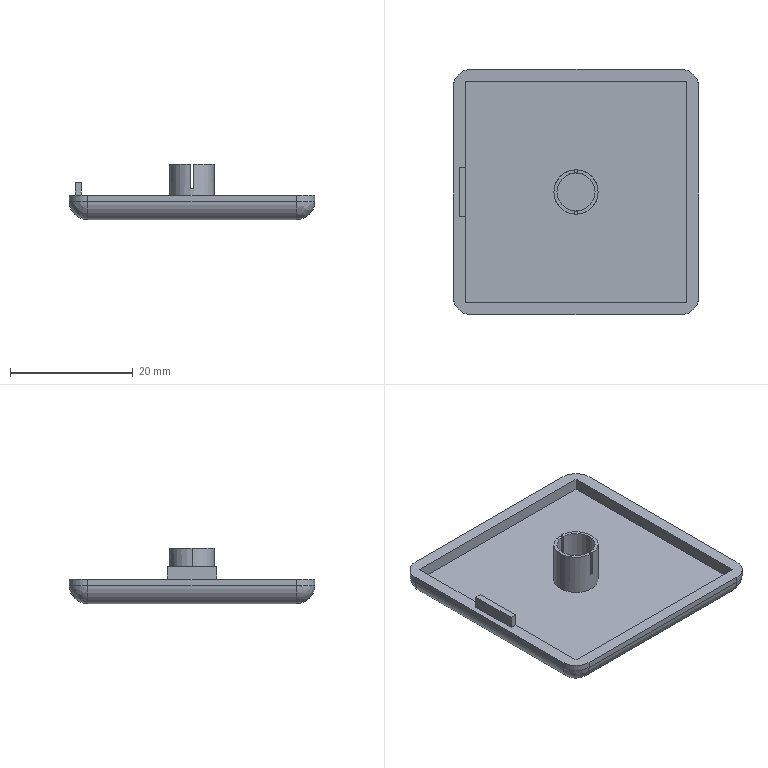Part | SolidWorks | features BaseBody 1 | 1 solid | 40 faces | box 40 x 40 x 9 mm | volume 3574 mm3 | plane 24 | cylinder 12 | spline 4 | commonest cylinder face diameters 6 x8 6.2 x2 7.2 x2
STEP:
#1=CARTESIAN_POINT('',(3.6,0.,-2.));
#2=VERTEX_POINT('',#1);
#3=CARTESIAN_POINT('',(-3.6,0.,-2.));
#4=VERTEX_POINT('',#3);
#5=CARTESIAN_POINT('',(0.,0.,-2.));
#6=DIRECTION('',(0.,0.,-1.));
#7=DIRECTION('',(-1.,0.,0.));
#8=AXIS2_PLACEMENT_3D('',#5,#6,#7);
#9=CIRCLE('',#8,3.6);
#10=EDGE_CURVE('',#2,#4,#9,.T.);
#11=ORIENTED_EDGE('',*,*,#10,.F.);
#12=CARTESIAN_POINT('',(3.6,0.,5.));
#13=VERTEX_POINT('',#12);
#14=CARTESIAN_POINT('',(3.6,0.,5.));
#15=DIRECTION('',(0.,0.,1.));
#16=VECTOR('',#15,1000.);
#17=LINE('',#14,#16);
#18=EDGE_CURVE('',#2,#13,#17,.T.);
#19=ORIENTED_EDGE('',*,*,#18,.T.);
#20=CARTESIAN_POINT('',(0.288,-3.588,5.));
#21=VERTEX_POINT('',#20);
#22=CARTESIAN_POINT('',(0.,0.,5.));
#23=DIRECTION('',(0.,0.,-1.));
#24=DIRECTION('',(-1.,0.,0.));
#25=AXIS2_PLACEMENT_3D('',#22,#23,#24);
#26=CIRCLE('',#25,3.6);
#27=EDGE_CURVE('',#13,#21,#26,.T.);
#28=ORIENTED_EDGE('',*,*,#27,.T.);
#29=CARTESIAN_POINT('',(0.288,-3.588,1.));
#30=VERTEX_POINT('',#29);
#31=CARTESIAN_POINT('',(0.288,-3.588,5.));
#32=DIRECTION('',(0.,0.,-1.));
#33=VECTOR('',#32,1000.);
#34=LINE('',#31,#33);
#35=EDGE_CURVE('',#21,#30,#34,.T.);
#36=ORIENTED_EDGE('',*,*,#35,.T.);
#37=CARTESIAN_POINT('',(-0.288,-3.588,1.));
#38=VERTEX_POINT('',#37);
#39=CARTESIAN_POINT('',(0.,0.,1.));
#40=DIRECTION('',(0.,0.,-1.));
#41=DIRECTION('',(-1.,0.,0.));
#42=AXIS2_PLACEMENT_3D('',#39,#40,#41);
#43=CIRCLE('',#42,3.6);
#44=EDGE_CURVE('',#30,#38,#43,.T.);
#45=ORIENTED_EDGE('',*,*,#44,.T.);
#46=CARTESIAN_POINT('',(-0.288,-3.588,5.));
#47=VERTEX_POINT('',#46);
#48=CARTESIAN_POINT('',(-0.288,-3.588,5.));
#49=DIRECTION('',(0.,0.,1.));
#50=VECTOR('',#49,1000.);
#51=LINE('',#48,#50);
#52=EDGE_CURVE('',#38,#47,#51,.T.);
#53=ORIENTED_EDGE('',*,*,#52,.T.);
#54=CARTESIAN_POINT('',(-3.6,0.,5.));
#55=VERTEX_POINT('',#54);
#56=CARTESIAN_POINT('',(0.,0.,5.));
#57=DIRECTION('',(0.,0.,-1.));
#58=DIRECTION('',(-1.,0.,0.));
#59=AXIS2_PLACEMENT_3D('',#56,#57,#58);
#60=CIRCLE('',#59,3.6);
#61=EDGE_CURVE('',#47,#55,#60,.T.);
#62=ORIENTED_EDGE('',*,*,#61,.T.);
#63=CARTESIAN_POINT('',(-3.6,0.,5.));
#64=DIRECTION('',(0.,0.,1.));
#65=VECTOR('',#64,1000.);
#66=LINE('',#63,#65);
#67=EDGE_CURVE('',#4,#55,#66,.T.);
#68=ORIENTED_EDGE('',*,*,#67,.F.);
#69=EDGE_LOOP('',(#11,#19,#28,#36,#45,#53,#62,#68));
#70=FACE_OUTER_BOUND('',#69,.T.);
#71=CARTESIAN_POINT('',(0.,0.,5.));
#72=DIRECTION('',(0.,0.,1.));
#73=DIRECTION('',(-1.,0.,0.));
#74=AXIS2_PLACEMENT_3D('',#71,#72,#73);
#75=CYLINDRICAL_SURFACE('',#74,3.6);
#76=ADVANCED_FACE('',(#70),#75,.T.);
#77=CARTESIAN_POINT('',(3.1,0.,-2.));
#78=VERTEX_POINT('',#77);
#79=CARTESIAN_POINT('',(-3.1,0.,-2.));
#80=VERTEX_POINT('',#79);
#81=CARTESIAN_POINT('',(0.,0.,-2.));
#82=DIRECTION('',(0.,0.,1.));
#83=DIRECTION('',(-1.,0.,0.));
#84=AXIS2_PLACEMENT_3D('',#81,#82,#83);
#85=CIRCLE('',#84,3.1);
#86=EDGE_CURVE('',#78,#80,#85,.T.);
#87=ORIENTED_EDGE('',*,*,#86,.F.);
#88=CARTESIAN_POINT('',(3.1,0.,5.));
#89=VERTEX_POINT('',#88);
#90=CARTESIAN_POINT('',(3.1,0.,5.));
#91=DIRECTION('',(0.,0.,1.));
#92=VECTOR('',#91,1000.);
#93=LINE('',#90,#92);
#94=EDGE_CURVE('',#78,#89,#93,.T.);
#95=ORIENTED_EDGE('',*,*,#94,.T.);
#96=CARTESIAN_POINT('',(0.288,3.087,5.));
#97=VERTEX_POINT('',#96);
#98=CARTESIAN_POINT('',(0.,0.,5.));
#99=DIRECTION('',(0.,0.,-1.));
#100=DIRECTION('',(-1.,0.,0.));
#101=AXIS2_PLACEMENT_3D('',#98,#99,#100);
#102=CIRCLE('',#101,3.1);
#103=EDGE_CURVE('',#97,#89,#102,.T.);
#104=ORIENTED_EDGE('',*,*,#103,.F.);
#105=CARTESIAN_POINT('',(0.288,3.087,1.));
#106=VERTEX_POINT('',#105);
#107=CARTESIAN_POINT('',(0.288,3.087,1.));
#108=DIRECTION('',(0.,0.,-1.));
#109=VECTOR('',#108,1000.);
#110=LINE('',#107,#109);
#111=EDGE_CURVE('',#97,#106,#110,.T.);
#112=ORIENTED_EDGE('',*,*,#111,.T.);
#113=CARTESIAN_POINT('',(-0.288,3.087,1.));
#114=VERTEX_POINT('',#113);
#115=CARTESIAN_POINT('',(0.,0.,1.));
#116=DIRECTION('',(0.,0.,-1.));
#117=DIRECTION('',(-1.,0.,0.));
#118=AXIS2_PLACEMENT_3D('',#115,#116,#117);
#119=CIRCLE('',#118,3.1);
#120=EDGE_CURVE('',#114,#106,#119,.T.);
#121=ORIENTED_EDGE('',*,*,#120,.F.);
#122=CARTESIAN_POINT('',(-0.288,3.087,5.));
#123=VERTEX_POINT('',#122);
#124=CARTESIAN_POINT('',(-0.288,3.087,1.));
#125=DIRECTION('',(0.,0.,1.));
#126=VECTOR('',#125,1000.);
#127=LINE('',#124,#126);
#128=EDGE_CURVE('',#114,#123,#127,.T.);
#129=ORIENTED_EDGE('',*,*,#128,.T.);
#130=CARTESIAN_POINT('',(-3.1,0.,5.));
#131=VERTEX_POINT('',#130);
#132=CARTESIAN_POINT('',(0.,0.,5.));
#133=DIRECTION('',(0.,0.,-1.));
#134=DIRECTION('',(-1.,0.,0.));
#135=AXIS2_PLACEMENT_3D('',#132,#133,#134);
#136=CIRCLE('',#135,3.1);
#137=EDGE_CURVE('',#131,#123,#136,.T.);
#138=ORIENTED_EDGE('',*,*,#137,.F.);
#139=CARTESIAN_POINT('',(-3.1,0.,5.));
#140=DIRECTION('',(0.,0.,1.));
#141=VECTOR('',#140,1000.);
#142=LINE('',#139,#141);
#143=EDGE_CURVE('',#80,#131,#142,.T.);
#144=ORIENTED_EDGE('',*,*,#143,.F.);
#145=EDGE_LOOP('',(#87,#95,#104,#112,#121,#129,#138,#144));
#146=FACE_OUTER_BOUND('',#145,.T.);
#147=CARTESIAN_POINT('',(0.,0.,5.));
#148=DIRECTION('',(0.,0.,1.));
#149=DIRECTION('',(-1.,0.,0.));
#150=AXIS2_PLACEMENT_3D('',#147,#148,#149);
#151=CYLINDRICAL_SURFACE('',#150,3.1);
#152=ADVANCED_FACE('',(#146),#151,.F.);
#153=CARTESIAN_POINT('',(-18.,-18.,-2.));
#154=VERTEX_POINT('',#153);
#155=CARTESIAN_POINT('',(18.,-18.,-2.));
#156=VERTEX_POINT('',#155);
#157=CARTESIAN_POINT('',(-20.,-18.,-2.));
#158=DIRECTION('',(1.,0.,0.));
#159=VECTOR('',#158,1000.);
#160=LINE('',#157,#159);
#161=EDGE_CURVE('',#154,#156,#160,.T.);
#162=ORIENTED_EDGE('',*,*,#161,.T.);
#163=CARTESIAN_POINT('',(18.,18.,-2.));
#164=VERTEX_POINT('',#163);
#165=CARTESIAN_POINT('',(18.,20.,-2.));
#166=DIRECTION('',(0.,1.,0.));
#167=VECTOR('',#166,1000.);
#168=LINE('',#165,#167);
#169=EDGE_CURVE('',#156,#164,#168,.T.);
#170=ORIENTED_EDGE('',*,*,#169,.T.);
#171=CARTESIAN_POINT('',(-18.,18.,-2.));
#172=VERTEX_POINT('',#171);
#173=CARTESIAN_POINT('',(-20.,18.,-2.));
#174=DIRECTION('',(-1.,0.,0.));
#175=VECTOR('',#174,1000.);
#176=LINE('',#173,#175);
#177=EDGE_CURVE('',#164,#172,#176,.T.);
#178=ORIENTED_EDGE('',*,*,#177,.T.);
#179=CARTESIAN_POINT('',(-18.,20.,-2.));
#180=DIRECTION('',(0.,-1.,0.));
#181=VECTOR('',#180,1000.);
#182=LINE('',#179,#181);
#183=EDGE_CURVE('',#172,#154,#182,.T.);
#184=ORIENTED_EDGE('',*,*,#183,.T.);
#185=EDGE_LOOP('',(#162,#170,#178,#184));
#186=FACE_OUTER_BOUND('',#185,.T.);
#187=CARTESIAN_POINT('',(0.,0.,-2.));
#188=DIRECTION('',(0.,0.,-1.));
#189=DIRECTION('',(-1.,0.,0.));
#190=AXIS2_PLACEMENT_3D('',#187,#188,#189);
#191=CIRCLE('',#190,3.6);
#192=EDGE_CURVE('',#4,#2,#191,.T.);
#193=ORIENTED_EDGE('',*,*,#192,.T.);
#194=ORIENTED_EDGE('',*,*,#10,.T.);
#195=EDGE_LOOP('',(#193,#194));
#196=FACE_BOUND('',#195,.T.);
#197=CARTESIAN_POINT('',(-20.,20.,-2.));
#198=DIRECTION('',(0.,0.,1.));
#199=DIRECTION('',(-1.,0.,0.));
#200=AXIS2_PLACEMENT_3D('',#197,#198,#199);
#201=PLANE('',#200);
#202=ADVANCED_FACE('',(#186,#196),#201,.T.);
#203=CARTESIAN_POINT('',(18.,18.,0.));
#204=VERTEX_POINT('',#203);
#205=CARTESIAN_POINT('',(18.,18.,-2.));
#206=DIRECTION('',(0.,0.,1.));
#207=VECTOR('',#206,1000.);
#208=LINE('',#205,#207);
#209=EDGE_CURVE('',#164,#204,#208,.T.);
#210=ORIENTED_EDGE('',*,*,#209,.F.);
#211=ORIENTED_EDGE('',*,*,#169,.F.);
#212=CARTESIAN_POINT('',(18.,-18.,0.));
#213=VERTEX_POINT('',#212);
#214=CARTESIAN_POINT('',(18.,-18.,-2.));
#215=DIRECTION('',(0.,0.,-1.));
#216=VECTOR('',#215,1000.);
#217=LINE('',#214,#216);
#218=EDGE_CURVE('',#213,#156,#217,.T.);
#219=ORIENTED_EDGE('',*,*,#218,.F.);
#220=CARTESIAN_POINT('',(18.,-18.,0.));
#221=DIRECTION('',(0.,-1.,0.));
#222=VECTOR('',#221,1000.);
#223=LINE('',#220,#222);
#224=EDGE_CURVE('',#204,#213,#223,.T.);
#225=ORIENTED_EDGE('',*,*,#224,.F.);
#226=EDGE_LOOP('',(#210,#211,#219,#225));
#227=FACE_OUTER_BOUND('',#226,.T.);
#228=CARTESIAN_POINT('',(18.,-18.,-2.));
#229=DIRECTION('',(1.,0.,0.));
#230=DIRECTION('',(0.,1.,0.));
#231=AXIS2_PLACEMENT_3D('',#228,#229,#230);
#232=PLANE('',#231);
#233=ADVANCED_FACE('',(#227),#232,.F.);
#234=ORIENTED_EDGE('',*,*,#218,.T.);
#235=ORIENTED_EDGE('',*,*,#161,.F.);
#236=CARTESIAN_POINT('',(-18.,-18.,0.));
#237=VERTEX_POINT('',#236);
#238=CARTESIAN_POINT('',(-18.,-18.,-2.));
#239=DIRECTION('',(0.,0.,-1.));
#240=VECTOR('',#239,1000.);
#241=LINE('',#238,#240);
#242=EDGE_CURVE('',#237,#154,#241,.T.);
#243=ORIENTED_EDGE('',*,*,#242,.F.);
#244=CARTESIAN_POINT('',(-18.,-18.,0.));
#245=DIRECTION('',(-1.,0.,0.));
#246=VECTOR('',#245,1000.);
#247=LINE('',#244,#246);
#248=EDGE_CURVE('',#213,#237,#247,.T.);
#249=ORIENTED_EDGE('',*,*,#248,.F.);
#250=EDGE_LOOP('',(#234,#235,#243,#249));
#251=FACE_OUTER_BOUND('',#250,.T.);
#252=CARTESIAN_POINT('',(-18.,-18.,-2.));
#253=DIRECTION('',(0.,-1.,0.));
#254=DIRECTION('',(1.,0.,0.));
#255=AXIS2_PLACEMENT_3D('',#252,#253,#254);
#256=PLANE('',#255);
#257=ADVANCED_FACE('',(#251),#256,.F.);
#258=CARTESIAN_POINT('',(-18.,4.05,2.));
#259=VERTEX_POINT('',#258);
#260=CARTESIAN_POINT('',(-18.,4.05,0.));
#261=VERTEX_POINT('',#260);
#262=CARTESIAN_POINT('',(-18.,4.05,-2.));
#263=DIRECTION('',(0.,0.,-1.));
#264=VECTOR('',#263,1000.);
#265=LINE('',#262,#264);
#266=EDGE_CURVE('',#259,#261,#265,.T.);
#267=ORIENTED_EDGE('',*,*,#266,.F.);
#268=CARTESIAN_POINT('',(-18.,-4.05,2.));
#269=VERTEX_POINT('',#268);
#270=CARTESIAN_POINT('',(-18.,18.,2.));
#271=DIRECTION('',(0.,1.,0.));
#272=VECTOR('',#271,1000.);
#273=LINE('',#270,#272);
#274=EDGE_CURVE('',#269,#259,#273,.T.);
#275=ORIENTED_EDGE('',*,*,#274,.F.);
#276=CARTESIAN_POINT('',(-18.,-4.05,0.));
#277=VERTEX_POINT('',#276);
#278=CARTESIAN_POINT('',(-18.,-4.05,-2.));
#279=DIRECTION('',(0.,0.,1.));
#280=VECTOR('',#279,1000.);
#281=LINE('',#278,#280);
#282=EDGE_CURVE('',#277,#269,#281,.T.);
#283=ORIENTED_EDGE('',*,*,#282,.F.);
#284=CARTESIAN_POINT('',(-18.,18.,0.));
#285=DIRECTION('',(0.,1.,0.));
#286=VECTOR('',#285,1000.);
#287=LINE('',#284,#286);
#288=EDGE_CURVE('',#237,#277,#287,.T.);
#289=ORIENTED_EDGE('',*,*,#288,.F.);
#290=ORIENTED_EDGE('',*,*,#242,.T.);
#291=ORIENTED_EDGE('',*,*,#183,.F.);
#292=CARTESIAN_POINT('',(-18.,18.,0.));
#293=VERTEX_POINT('',#292);
#294=CARTESIAN_POINT('',(-18.,18.,-2.));
#295=DIRECTION('',(0.,0.,-1.));
#296=VECTOR('',#295,1000.);
#297=LINE('',#294,#296);
#298=EDGE_CURVE('',#293,#172,#297,.T.);
#299=ORIENTED_EDGE('',*,*,#298,.F.);
#300=CARTESIAN_POINT('',(-18.,18.,0.));
#301=DIRECTION('',(0.,1.,0.));
#302=VECTOR('',#301,1000.);
#303=LINE('',#300,#302);
#304=EDGE_CURVE('',#261,#293,#303,.T.);
#305=ORIENTED_EDGE('',*,*,#304,.F.);
#306=EDGE_LOOP('',(#267,#275,#283,#289,#290,#291,#299,#305));
#307=FACE_OUTER_BOUND('',#306,.T.);
#308=CARTESIAN_POINT('',(-18.,18.,-2.));
#309=DIRECTION('',(-1.,0.,0.));
#310=DIRECTION('',(0.,-1.,0.));
#311=AXIS2_PLACEMENT_3D('',#308,#309,#310);
#312=PLANE('',#311);
#313=ADVANCED_FACE('',(#307),#312,.F.);
#314=ORIENTED_EDGE('',*,*,#298,.T.);
#315=ORIENTED_EDGE('',*,*,#177,.F.);
#316=ORIENTED_EDGE('',*,*,#209,.T.);
#317=CARTESIAN_POINT('',(18.,18.,0.));
#318=DIRECTION('',(1.,0.,0.));
#319=VECTOR('',#318,1000.);
#320=LINE('',#317,#319);
#321=EDGE_CURVE('',#293,#204,#320,.T.);
#322=ORIENTED_EDGE('',*,*,#321,.F.);
#323=EDGE_LOOP('',(#314,#315,#316,#322));
#324=FACE_OUTER_BOUND('',#323,.T.);
#325=CARTESIAN_POINT('',(18.,18.,-2.));
#326=DIRECTION('',(0.,1.,0.));
#327=DIRECTION('',(-1.,0.,0.));
#328=AXIS2_PLACEMENT_3D('',#325,#326,#327);
#329=PLANE('',#328);
#330=ADVANCED_FACE('',(#324),#329,.F.);
#331=ORIENTED_EDGE('',*,*,#18,.F.);
#332=ORIENTED_EDGE('',*,*,#192,.F.);
#333=ORIENTED_EDGE('',*,*,#67,.T.);
#334=CARTESIAN_POINT('',(-0.288,3.588,5.));
#335=VERTEX_POINT('',#334);
#336=CARTESIAN_POINT('',(0.,0.,5.));
#337=DIRECTION('',(0.,0.,-1.));
#338=DIRECTION('',(-1.,0.,0.));
#339=AXIS2_PLACEMENT_3D('',#336,#337,#338);
#340=CIRCLE('',#339,3.6);
#341=EDGE_CURVE('',#55,#335,#340,.T.);
#342=ORIENTED_EDGE('',*,*,#341,.T.);
#343=CARTESIAN_POINT('',(-0.288,3.588,1.));
#344=VERTEX_POINT('',#343);
#345=CARTESIAN_POINT('',(-0.288,3.588,5.));
#346=DIRECTION('',(0.,0.,-1.));
#347=VECTOR('',#346,1000.);
#348=LINE('',#345,#347);
#349=EDGE_CURVE('',#335,#344,#348,.T.);
#350=ORIENTED_EDGE('',*,*,#349,.T.);
#351=CARTESIAN_POINT('',(0.288,3.588,1.));
#352=VERTEX_POINT('',#351);
#353=CARTESIAN_POINT('',(0.,0.,1.));
#354=DIRECTION('',(0.,0.,-1.));
#355=DIRECTION('',(-1.,0.,0.));
#356=AXIS2_PLACEMENT_3D('',#353,#354,#355);
#357=CIRCLE('',#356,3.6);
#358=EDGE_CURVE('',#344,#352,#357,.T.);
#359=ORIENTED_EDGE('',*,*,#358,.T.);
#360=CARTESIAN_POINT('',(0.288,3.588,5.));
#361=VERTEX_POINT('',#360);
#362=CARTESIAN_POINT('',(0.288,3.588,5.));
#363=DIRECTION('',(0.,0.,1.));
#364=VECTOR('',#363,1000.);
#365=LINE('',#362,#364);
#366=EDGE_CURVE('',#352,#361,#365,.T.);
#367=ORIENTED_EDGE('',*,*,#366,.T.);
#368=CARTESIAN_POINT('',(0.,0.,5.));
#369=DIRECTION('',(0.,0.,-1.));
#370=DIRECTION('',(-1.,0.,0.));
#371=AXIS2_PLACEMENT_3D('',#368,#369,#370);
#372=CIRCLE('',#371,3.6);
#373=EDGE_CURVE('',#361,#13,#372,.T.);
#374=ORIENTED_EDGE('',*,*,#373,.T.);
#375=EDGE_LOOP('',(#331,#332,#333,#342,#350,#359,#367,#374));
#376=FACE_OUTER_BOUND('',#375,.T.);
#377=CARTESIAN_POINT('',(0.,0.,5.));
#378=DIRECTION('',(0.,0.,1.));
#379=DIRECTION('',(-1.,0.,0.));
#380=AXIS2_PLACEMENT_3D('',#377,#378,#379);
#381=CYLINDRICAL_SURFACE('',#380,3.6);
#382=ADVANCED_FACE('',(#376),#381,.T.);
#383=CARTESIAN_POINT('',(20.,-17.,0.));
#384=VERTEX_POINT('',#383);
#385=CARTESIAN_POINT('',(20.,17.,0.));
#386=VERTEX_POINT('',#385);
#387=CARTESIAN_POINT('',(20.,17.,0.));
#388=DIRECTION('',(0.,1.,0.));
#389=VECTOR('',#388,1000.);
#390=LINE('',#387,#389);
#391=EDGE_CURVE('',#384,#386,#390,.T.);
#392=ORIENTED_EDGE('',*,*,#391,.T.);
#393=CARTESIAN_POINT('',(17.,20.,0.));
#394=VERTEX_POINT('',#393);
#395=CARTESIAN_POINT('',(17.,17.,0.));
#396=DIRECTION('',(0.,0.,1.));
#397=DIRECTION('',(1.,0.,0.));
#398=AXIS2_PLACEMENT_3D('',#395,#396,#397);
#399=CIRCLE('',#398,3.);
#400=EDGE_CURVE('',#386,#394,#399,.T.);
#401=ORIENTED_EDGE('',*,*,#400,.T.);
#402=CARTESIAN_POINT('',(-17.,20.,0.));
#403=VERTEX_POINT('',#402);
#404=CARTESIAN_POINT('',(-17.,20.,0.));
#405=DIRECTION('',(-1.,0.,0.));
#406=VECTOR('',#405,1000.);
#407=LINE('',#404,#406);
#408=EDGE_CURVE('',#394,#403,#407,.T.);
#409=ORIENTED_EDGE('',*,*,#408,.T.);
#410=CARTESIAN_POINT('',(-20.,17.,0.));
#411=VERTEX_POINT('',#410);
#412=CARTESIAN_POINT('',(-17.,17.,0.));
#413=DIRECTION('',(0.,0.,1.));
#414=DIRECTION('',(1.,0.,0.));
#415=AXIS2_PLACEMENT_3D('',#412,#413,#414);
#416=CIRCLE('',#415,3.);
#417=EDGE_CURVE('',#403,#411,#416,.T.);
#418=ORIENTED_EDGE('',*,*,#417,.T.);
#419=CARTESIAN_POINT('',(-20.,-17.,0.));
#420=VERTEX_POINT('',#419);
#421=CARTESIAN_POINT('',(-20.,17.,0.));
#422=DIRECTION('',(0.,-1.,0.));
#423=VECTOR('',#422,1000.);
#424=LINE('',#421,#423);
#425=EDGE_CURVE('',#411,#420,#424,.T.);
#426=ORIENTED_EDGE('',*,*,#425,.T.);
#427=CARTESIAN_POINT('',(-17.,-20.,0.));
#428=VERTEX_POINT('',#427);
#429=CARTESIAN_POINT('',(-17.,-17.,0.));
#430=DIRECTION('',(0.,0.,1.));
#431=DIRECTION('',(1.,0.,0.));
#432=AXIS2_PLACEMENT_3D('',#429,#430,#431);
#433=CIRCLE('',#432,3.);
#434=EDGE_CURVE('',#420,#428,#433,.T.);
#435=ORIENTED_EDGE('',*,*,#434,.T.);
#436=CARTESIAN_POINT('',(17.,-20.,0.));
#437=VERTEX_POINT('',#436);
#438=CARTESIAN_POINT('',(-17.,-20.,0.));
#439=DIRECTION('',(1.,0.,0.));
#440=VECTOR('',#439,1000.);
#441=LINE('',#438,#440);
#442=EDGE_CURVE('',#428,#437,#441,.T.);
#443=ORIENTED_EDGE('',*,*,#442,.T.);
#444=CARTESIAN_POINT('',(17.,-17.,0.));
#445=DIRECTION('',(0.,0.,1.));
#446=DIRECTION('',(1.,0.,0.));
#447=AXIS2_PLACEMENT_3D('',#444,#445,#446);
#448=CIRCLE('',#447,3.);
#449=EDGE_CURVE('',#437,#384,#448,.T.);
#450=ORIENTED_EDGE('',*,*,#449,.T.);
#451=EDGE_LOOP('',(#392,#401,#409,#418,#426,#435,#443,#450));
#452=FACE_OUTER_BOUND('',#451,.T.);
#453=CARTESIAN_POINT('',(-19.,-4.05,0.));
#454=VERTEX_POINT('',#453);
#455=CARTESIAN_POINT('',(-17.,-4.05,0.));
#456=DIRECTION('',(-1.,0.,0.));
#457=VECTOR('',#456,1000.);
#458=LINE('',#455,#457);
#459=EDGE_CURVE('',#277,#454,#458,.T.);
#460=ORIENTED_EDGE('',*,*,#459,.T.);
#461=CARTESIAN_POINT('',(-19.,4.05,0.));
#462=VERTEX_POINT('',#461);
#463=CARTESIAN_POINT('',(-19.,17.,0.));
#464=DIRECTION('',(0.,1.,0.));
#465=VECTOR('',#464,1000.);
#466=LINE('',#463,#465);
#467=EDGE_CURVE('',#454,#462,#466,.T.);
#468=ORIENTED_EDGE('',*,*,#467,.T.);
#469=CARTESIAN_POINT('',(-17.,4.05,0.));
#470=DIRECTION('',(1.,0.,0.));
#471=VECTOR('',#470,1000.);
#472=LINE('',#469,#471);
#473=EDGE_CURVE('',#462,#261,#472,.T.);
#474=ORIENTED_EDGE('',*,*,#473,.T.);
#475=ORIENTED_EDGE('',*,*,#304,.T.);
#476=ORIENTED_EDGE('',*,*,#321,.T.);
#477=ORIENTED_EDGE('',*,*,#224,.T.);
#478=ORIENTED_EDGE('',*,*,#248,.T.);
#479=ORIENTED_EDGE('',*,*,#288,.T.);
#480=EDGE_LOOP('',(#460,#468,#474,#475,#476,#477,#478,#479));
#481=FACE_BOUND('',#480,.T.);
#482=CARTESIAN_POINT('',(-17.,17.,0.));
#483=DIRECTION('',(0.,0.,1.));
#484=DIRECTION('',(-1.,0.,0.));
#485=AXIS2_PLACEMENT_3D('',#482,#483,#484);
#486=PLANE('',#485);
#487=ADVANCED_FACE('',(#452,#481),#486,.T.);
#488=CARTESIAN_POINT('',(-19.,4.05,2.));
#489=VERTEX_POINT('',#488);
#490=CARTESIAN_POINT('',(-19.,4.05,2.));
#491=DIRECTION('',(0.,0.,-1.));
#492=VECTOR('',#491,1000.);
#493=LINE('',#490,#492);
#494=EDGE_CURVE('',#489,#462,#493,.T.);
#495=ORIENTED_EDGE('',*,*,#494,.F.);
#496=CARTESIAN_POINT('',(-18.,4.05,2.));
#497=DIRECTION('',(-1.,0.,0.));
#498=VECTOR('',#497,1000.);
#499=LINE('',#496,#498);
#500=EDGE_CURVE('',#259,#489,#499,.T.);
#501=ORIENTED_EDGE('',*,*,#500,.F.);
#502=ORIENTED_EDGE('',*,*,#266,.T.);
#503=ORIENTED_EDGE('',*,*,#473,.F.);
#504=EDGE_LOOP('',(#495,#501,#502,#503));
#505=FACE_OUTER_BOUND('',#504,.T.);
#506=CARTESIAN_POINT('',(-18.,4.05,2.));
#507=DIRECTION('',(0.,-1.,0.));
#508=DIRECTION('',(1.,0.,0.));
#509=AXIS2_PLACEMENT_3D('',#506,#507,#508);
#510=PLANE('',#509);
#511=ADVANCED_FACE('',(#505),#510,.F.);
#512=CARTESIAN_POINT('',(-19.,-4.05,2.));
#513=VERTEX_POINT('',#512);
#514=CARTESIAN_POINT('',(-20.,-4.05,2.));
#515=DIRECTION('',(1.,0.,0.));
#516=VECTOR('',#515,1000.);
#517=LINE('',#514,#516);
#518=EDGE_CURVE('',#513,#269,#517,.T.);
#519=ORIENTED_EDGE('',*,*,#518,.T.);
#520=ORIENTED_EDGE('',*,*,#274,.T.);
#521=ORIENTED_EDGE('',*,*,#500,.T.);
#522=CARTESIAN_POINT('',(-19.,20.,2.));
#523=DIRECTION('',(0.,-1.,0.));
#524=VECTOR('',#523,1000.);
#525=LINE('',#522,#524);
#526=EDGE_CURVE('',#489,#513,#525,.T.);
#527=ORIENTED_EDGE('',*,*,#526,.T.);
#528=EDGE_LOOP('',(#519,#520,#521,#527));
#529=FACE_OUTER_BOUND('',#528,.T.);
#530=CARTESIAN_POINT('',(-20.,20.,2.));
#531=DIRECTION('',(0.,0.,1.));
#532=DIRECTION('',(-1.,0.,0.));
#533=AXIS2_PLACEMENT_3D('',#530,#531,#532);
#534=PLANE('',#533);
#535=ADVANCED_FACE('',(#529),#534,.T.);
#536=ORIENTED_EDGE('',*,*,#282,.T.);
#537=ORIENTED_EDGE('',*,*,#518,.F.);
#538=CARTESIAN_POINT('',(-19.,-4.05,2.));
#539=DIRECTION('',(0.,0.,1.));
#540=VECTOR('',#539,1000.);
#541=LINE('',#538,#540);
#542=EDGE_CURVE('',#454,#513,#541,.T.);
#543=ORIENTED_EDGE('',*,*,#542,.F.);
#544=ORIENTED_EDGE('',*,*,#459,.F.);
#545=EDGE_LOOP('',(#536,#537,#543,#544));
#546=FACE_OUTER_BOUND('',#545,.T.);
#547=CARTESIAN_POINT('',(-19.,-4.05,2.));
#548=DIRECTION('',(0.,1.,0.));
#549=DIRECTION('',(-1.,0.,0.));
#550=AXIS2_PLACEMENT_3D('',#547,#548,#549);
#551=PLANE('',#550);
#552=ADVANCED_FACE('',(#546),#551,.F.);
#553=CARTESIAN_POINT('',(0.288,-3.588,5.));
#554=DIRECTION('',(0.,-1.,0.));
#555=VECTOR('',#554,1000.);
#556=LINE('',#553,#555);
#557=EDGE_CURVE('',#361,#97,#556,.T.);
#558=ORIENTED_EDGE('',*,*,#557,.F.);
#559=ORIENTED_EDGE('',*,*,#366,.F.);
#560=CARTESIAN_POINT('',(0.288,-3.588,1.));
#561=DIRECTION('',(0.,1.,0.));
#562=VECTOR('',#561,1000.);
#563=LINE('',#560,#562);
#564=EDGE_CURVE('',#106,#352,#563,.T.);
#565=ORIENTED_EDGE('',*,*,#564,.F.);
#566=ORIENTED_EDGE('',*,*,#111,.F.);
#567=EDGE_LOOP('',(#558,#559,#565,#566));
#568=FACE_OUTER_BOUND('',#567,.T.);
#569=CARTESIAN_POINT('',(0.288,-3.588,1.));
#570=DIRECTION('',(1.,0.,0.));
#571=DIRECTION('',(0.,1.,0.));
#572=AXIS2_PLACEMENT_3D('',#569,#570,#571);
#573=PLANE('',#572);
#574=ADVANCED_FACE('',(#568),#573,.F.);
#575=CARTESIAN_POINT('',(-0.288,0.,1.));
#576=DIRECTION('',(0.,-1.,0.));
#577=VECTOR('',#576,1000.);
#578=LINE('',#575,#577);
#579=EDGE_CURVE('',#344,#114,#578,.T.);
#580=ORIENTED_EDGE('',*,*,#579,.T.);
#581=ORIENTED_EDGE('',*,*,#120,.T.);
#582=ORIENTED_EDGE('',*,*,#564,.T.);
#583=ORIENTED_EDGE('',*,*,#358,.F.);
#584=EDGE_LOOP('',(#580,#581,#582,#583));
#585=FACE_OUTER_BOUND('',#584,.T.);
#586=CARTESIAN_POINT('',(0.,0.,1.));
#587=DIRECTION('',(0.,0.,1.));
#588=DIRECTION('',(-1.,0.,0.));
#589=AXIS2_PLACEMENT_3D('',#586,#587,#588);
#590=PLANE('',#589);
#591=ADVANCED_FACE('',(#585),#590,.T.);
#592=ORIENTED_EDGE('',*,*,#579,.F.);
#593=ORIENTED_EDGE('',*,*,#349,.F.);
#594=CARTESIAN_POINT('',(-0.288,3.588,5.));
#595=DIRECTION('',(0.,1.,0.));
#596=VECTOR('',#595,1000.);
#597=LINE('',#594,#596);
#598=EDGE_CURVE('',#123,#335,#597,.T.);
#599=ORIENTED_EDGE('',*,*,#598,.F.);
#600=ORIENTED_EDGE('',*,*,#128,.F.);
#601=EDGE_LOOP('',(#592,#593,#599,#600));
#602=FACE_OUTER_BOUND('',#601,.T.);
#603=CARTESIAN_POINT('',(-0.288,3.588,1.));
#604=DIRECTION('',(-1.,0.,0.));
#605=DIRECTION('',(0.,-1.,0.));
#606=AXIS2_PLACEMENT_3D('',#603,#604,#605);
#607=PLANE('',#606);
#608=ADVANCED_FACE('',(#602),#607,.F.);
#609=CARTESIAN_POINT('',(-0.288,-3.087,5.));
#610=VERTEX_POINT('',#609);
#611=CARTESIAN_POINT('',(-0.288,0.,5.));
#612=DIRECTION('',(0.,1.,0.));
#613=VECTOR('',#612,1000.);
#614=LINE('',#611,#613);
#615=EDGE_CURVE('',#47,#610,#614,.T.);
#616=ORIENTED_EDGE('',*,*,#615,.T.);
#617=CARTESIAN_POINT('',(0.,0.,5.));
#618=DIRECTION('',(0.,0.,-1.));
#619=DIRECTION('',(-1.,0.,0.));
#620=AXIS2_PLACEMENT_3D('',#617,#618,#619);
#621=CIRCLE('',#620,3.1);
#622=EDGE_CURVE('',#610,#131,#621,.T.);
#623=ORIENTED_EDGE('',*,*,#622,.T.);
#624=ORIENTED_EDGE('',*,*,#137,.T.);
#625=ORIENTED_EDGE('',*,*,#598,.T.);
#626=ORIENTED_EDGE('',*,*,#341,.F.);
#627=ORIENTED_EDGE('',*,*,#61,.F.);
#628=EDGE_LOOP('',(#616,#623,#624,#625,#626,#627));
#629=FACE_OUTER_BOUND('',#628,.T.);
#630=CARTESIAN_POINT('',(0.,0.,5.));
#631=DIRECTION('',(0.,0.,1.));
#632=DIRECTION('',(-1.,0.,0.));
#633=AXIS2_PLACEMENT_3D('',#630,#631,#632);
#634=PLANE('',#633);
#635=ADVANCED_FACE('',(#629),#634,.T.);
#636=ORIENTED_EDGE('',*,*,#615,.F.);
#637=ORIENTED_EDGE('',*,*,#52,.F.);
#638=CARTESIAN_POINT('',(-0.288,-3.087,1.));
#639=VERTEX_POINT('',#638);
#640=CARTESIAN_POINT('',(-0.288,3.588,1.));
#641=DIRECTION('',(0.,-1.,0.));
#642=VECTOR('',#641,1000.);
#643=LINE('',#640,#642);
#644=EDGE_CURVE('',#639,#38,#643,.T.);
#645=ORIENTED_EDGE('',*,*,#644,.F.);
#646=CARTESIAN_POINT('',(-0.288,-3.087,1.));
#647=DIRECTION('',(0.,0.,-1.));
#648=VECTOR('',#647,1000.);
#649=LINE('',#646,#648);
#650=EDGE_CURVE('',#610,#639,#649,.T.);
#651=ORIENTED_EDGE('',*,*,#650,.F.);
#652=EDGE_LOOP('',(#636,#637,#645,#651));
#653=FACE_OUTER_BOUND('',#652,.T.);
#654=CARTESIAN_POINT('',(-0.288,3.588,1.));
#655=DIRECTION('',(-1.,0.,0.));
#656=DIRECTION('',(0.,-1.,0.));
#657=AXIS2_PLACEMENT_3D('',#654,#655,#656);
#658=PLANE('',#657);
#659=ADVANCED_FACE('',(#653),#658,.F.);
#660=CARTESIAN_POINT('',(0.288,-3.087,1.));
#661=VERTEX_POINT('',#660);
#662=CARTESIAN_POINT('',(0.288,0.,1.));
#663=DIRECTION('',(0.,1.,0.));
#664=VECTOR('',#663,1000.);
#665=LINE('',#662,#664);
#666=EDGE_CURVE('',#30,#661,#665,.T.);
#667=ORIENTED_EDGE('',*,*,#666,.T.);
#668=CARTESIAN_POINT('',(0.,0.,1.));
#669=DIRECTION('',(0.,0.,-1.));
#670=DIRECTION('',(-1.,0.,0.));
#671=AXIS2_PLACEMENT_3D('',#668,#669,#670);
#672=CIRCLE('',#671,3.1);
#673=EDGE_CURVE('',#661,#639,#672,.T.);
#674=ORIENTED_EDGE('',*,*,#673,.T.);
#675=ORIENTED_EDGE('',*,*,#644,.T.);
#676=ORIENTED_EDGE('',*,*,#44,.F.);
#677=EDGE_LOOP('',(#667,#674,#675,#676));
#678=FACE_OUTER_BOUND('',#677,.T.);
#679=CARTESIAN_POINT('',(0.,0.,1.));
#680=DIRECTION('',(0.,0.,1.));
#681=DIRECTION('',(-1.,0.,0.));
#682=AXIS2_PLACEMENT_3D('',#679,#680,#681);
#683=PLANE('',#682);
#684=ADVANCED_FACE('',(#678),#683,.T.);
#685=ORIENTED_EDGE('',*,*,#666,.F.);
#686=ORIENTED_EDGE('',*,*,#35,.F.);
#687=CARTESIAN_POINT('',(0.288,-3.087,5.));
#688=VERTEX_POINT('',#687);
#689=CARTESIAN_POINT('',(0.288,-3.588,5.));
#690=DIRECTION('',(0.,-1.,0.));
#691=VECTOR('',#690,1000.);
#692=LINE('',#689,#691);
#693=EDGE_CURVE('',#688,#21,#692,.T.);
#694=ORIENTED_EDGE('',*,*,#693,.F.);
#695=CARTESIAN_POINT('',(0.288,-3.087,1.));
#696=DIRECTION('',(0.,0.,1.));
#697=VECTOR('',#696,1000.);
#698=LINE('',#695,#697);
#699=EDGE_CURVE('',#661,#688,#698,.T.);
#700=ORIENTED_EDGE('',*,*,#699,.F.);
#701=EDGE_LOOP('',(#685,#686,#694,#700));
#702=FACE_OUTER_BOUND('',#701,.T.);
#703=CARTESIAN_POINT('',(0.288,-3.588,1.));
#704=DIRECTION('',(1.,0.,0.));
#705=DIRECTION('',(0.,1.,0.));
#706=AXIS2_PLACEMENT_3D('',#703,#704,#705);
#707=PLANE('',#706);
#708=ADVANCED_FACE('',(#702),#707,.F.);
#709=ORIENTED_EDGE('',*,*,#557,.T.);
#710=ORIENTED_EDGE('',*,*,#103,.T.);
#711=CARTESIAN_POINT('',(0.,0.,5.));
#712=DIRECTION('',(0.,0.,-1.));
#713=DIRECTION('',(-1.,0.,0.));
#714=AXIS2_PLACEMENT_3D('',#711,#712,#713);
#715=CIRCLE('',#714,3.1);
#716=EDGE_CURVE('',#89,#688,#715,.T.);
#717=ORIENTED_EDGE('',*,*,#716,.T.);
#718=ORIENTED_EDGE('',*,*,#693,.T.);
#719=ORIENTED_EDGE('',*,*,#27,.F.);
#720=ORIENTED_EDGE('',*,*,#373,.F.);
#721=EDGE_LOOP('',(#709,#710,#717,#718,#719,#720));
#722=FACE_OUTER_BOUND('',#721,.T.);
#723=CARTESIAN_POINT('',(0.,0.,5.));
#724=DIRECTION('',(0.,0.,1.));
#725=DIRECTION('',(-1.,0.,0.));
#726=AXIS2_PLACEMENT_3D('',#723,#724,#725);
#727=PLANE('',#726);
#728=ADVANCED_FACE('',(#722),#727,.T.);
#729=CARTESIAN_POINT('',(17.,20.,-1.));
#730=VERTEX_POINT('',#729);
#731=CARTESIAN_POINT('',(17.,20.,-4.));
#732=DIRECTION('',(0.,0.,1.));
#733=VECTOR('',#732,1000.);
#734=LINE('',#731,#733);
#735=EDGE_CURVE('',#730,#394,#734,.T.);
#736=ORIENTED_EDGE('',*,*,#735,.T.);
#737=ORIENTED_EDGE('',*,*,#400,.F.);
#738=CARTESIAN_POINT('',(20.,17.,-1.));
#739=VERTEX_POINT('',#738);
#740=CARTESIAN_POINT('',(20.,17.,-4.));
#741=DIRECTION('',(0.,0.,-1.));
#742=VECTOR('',#741,1000.);
#743=LINE('',#740,#742);
#744=EDGE_CURVE('',#386,#739,#743,.T.);
#745=ORIENTED_EDGE('',*,*,#744,.T.);
#746=CARTESIAN_POINT('',(17.,17.,-1.));
#747=DIRECTION('',(0.,0.,1.));
#748=DIRECTION('',(1.,0.,0.));
#749=AXIS2_PLACEMENT_3D('',#746,#747,#748);
#750=CIRCLE('',#749,3.);
#751=EDGE_CURVE('',#739,#730,#750,.T.);
#752=ORIENTED_EDGE('',*,*,#751,.T.);
#753=EDGE_LOOP('',(#736,#737,#745,#752));
#754=FACE_OUTER_BOUND('',#753,.T.);
#755=CARTESIAN_POINT('',(17.,17.,-4.));
#756=DIRECTION('',(0.,0.,-1.));
#757=DIRECTION('',(1.,0.,0.));
#758=AXIS2_PLACEMENT_3D('',#755,#756,#757);
#759=CYLINDRICAL_SURFACE('',#758,3.);
#760=ADVANCED_FACE('',(#754),#759,.T.);
#761=ORIENTED_EDGE('',*,*,#744,.F.);
#762=ORIENTED_EDGE('',*,*,#391,.F.);
#763=CARTESIAN_POINT('',(20.,-17.,-1.));
#764=VERTEX_POINT('',#763);
#765=CARTESIAN_POINT('',(20.,-17.,-4.));
#766=DIRECTION('',(0.,0.,-1.));
#767=VECTOR('',#766,1000.);
#768=LINE('',#765,#767);
#769=EDGE_CURVE('',#384,#764,#768,.T.);
#770=ORIENTED_EDGE('',*,*,#769,.T.);
#771=CARTESIAN_POINT('',(20.,-17.,-1.));
#772=DIRECTION('',(0.,1.,0.));
#773=VECTOR('',#772,1000.);
#774=LINE('',#771,#773);
#775=EDGE_CURVE('',#764,#739,#774,.T.);
#776=ORIENTED_EDGE('',*,*,#775,.T.);
#777=EDGE_LOOP('',(#761,#762,#770,#776));
#778=FACE_OUTER_BOUND('',#777,.T.);
#779=CARTESIAN_POINT('',(20.,-17.,-4.));
#780=DIRECTION('',(1.,0.,0.));
#781=DIRECTION('',(0.,1.,0.));
#782=AXIS2_PLACEMENT_3D('',#779,#780,#781);
#783=PLANE('',#782);
#784=ADVANCED_FACE('',(#778),#783,.T.);
#785=ORIENTED_EDGE('',*,*,#769,.F.);
#786=ORIENTED_EDGE('',*,*,#449,.F.);
#787=CARTESIAN_POINT('',(17.,-20.,-1.));
#788=VERTEX_POINT('',#787);
#789=CARTESIAN_POINT('',(17.,-20.,-4.));
#790=DIRECTION('',(0.,0.,-1.));
#791=VECTOR('',#790,1000.);
#792=LINE('',#789,#791);
#793=EDGE_CURVE('',#437,#788,#792,.T.);
#794=ORIENTED_EDGE('',*,*,#793,.T.);
#795=CARTESIAN_POINT('',(17.,-17.,-1.));
#796=DIRECTION('',(0.,0.,1.));
#797=DIRECTION('',(1.,0.,0.));
#798=AXIS2_PLACEMENT_3D('',#795,#796,#797);
#799=CIRCLE('',#798,3.);
#800=EDGE_CURVE('',#788,#764,#799,.T.);
#801=ORIENTED_EDGE('',*,*,#800,.T.);
#802=EDGE_LOOP('',(#785,#786,#794,#801));
#803=FACE_OUTER_BOUND('',#802,.T.);
#804=CARTESIAN_POINT('',(17.,-17.,-4.));
#805=DIRECTION('',(0.,0.,-1.));
#806=DIRECTION('',(1.,0.,0.));
#807=AXIS2_PLACEMENT_3D('',#804,#805,#806);
#808=CYLINDRICAL_SURFACE('',#807,3.);
#809=ADVANCED_FACE('',(#803),#808,.T.);
#810=ORIENTED_EDGE('',*,*,#793,.F.);
#811=ORIENTED_EDGE('',*,*,#442,.F.);
#812=CARTESIAN_POINT('',(-17.,-20.,-1.));
#813=VERTEX_POINT('',#812);
#814=CARTESIAN_POINT('',(-17.,-20.,-4.));
#815=DIRECTION('',(0.,0.,-1.));
#816=VECTOR('',#815,1000.);
#817=LINE('',#814,#816);
#818=EDGE_CURVE('',#428,#813,#817,.T.);
#819=ORIENTED_EDGE('',*,*,#818,.T.);
#820=CARTESIAN_POINT('',(-17.,-20.,-1.));
#821=DIRECTION('',(1.,0.,0.));
#822=VECTOR('',#821,1000.);
#823=LINE('',#820,#822);
#824=EDGE_CURVE('',#813,#788,#823,.T.);
#825=ORIENTED_EDGE('',*,*,#824,.T.);
#826=EDGE_LOOP('',(#810,#811,#819,#825));
#827=FACE_OUTER_BOUND('',#826,.T.);
#828=CARTESIAN_POINT('',(-17.,-20.,-4.));
#829=DIRECTION('',(0.,-1.,0.));
#830=DIRECTION('',(1.,0.,0.));
#831=AXIS2_PLACEMENT_3D('',#828,#829,#830);
#832=PLANE('',#831);
#833=ADVANCED_FACE('',(#827),#832,.T.);
#834=ORIENTED_EDGE('',*,*,#818,.F.);
#835=ORIENTED_EDGE('',*,*,#434,.F.);
#836=CARTESIAN_POINT('',(-20.,-17.,-1.));
#837=VERTEX_POINT('',#836);
#838=CARTESIAN_POINT('',(-20.,-17.,-4.));
#839=DIRECTION('',(0.,0.,-1.));
#840=VECTOR('',#839,1000.);
#841=LINE('',#838,#840);
#842=EDGE_CURVE('',#420,#837,#841,.T.);
#843=ORIENTED_EDGE('',*,*,#842,.T.);
#844=CARTESIAN_POINT('',(-17.,-17.,-1.));
#845=DIRECTION('',(0.,0.,1.));
#846=DIRECTION('',(1.,0.,0.));
#847=AXIS2_PLACEMENT_3D('',#844,#845,#846);
#848=CIRCLE('',#847,3.);
#849=EDGE_CURVE('',#837,#813,#848,.T.);
#850=ORIENTED_EDGE('',*,*,#849,.T.);
#851=EDGE_LOOP('',(#834,#835,#843,#850));
#852=FACE_OUTER_BOUND('',#851,.T.);
#853=CARTESIAN_POINT('',(-17.,-17.,-4.));
#854=DIRECTION('',(0.,0.,-1.));
#855=DIRECTION('',(1.,0.,0.));
#856=AXIS2_PLACEMENT_3D('',#853,#854,#855);
#857=CYLINDRICAL_SURFACE('',#856,3.);
#858=ADVANCED_FACE('',(#852),#857,.T.);
#859=ORIENTED_EDGE('',*,*,#842,.F.);
#860=ORIENTED_EDGE('',*,*,#425,.F.);
#861=CARTESIAN_POINT('',(-20.,17.,-1.));
#862=VERTEX_POINT('',#861);
#863=CARTESIAN_POINT('',(-20.,17.,-4.));
#864=DIRECTION('',(0.,0.,-1.));
#865=VECTOR('',#864,1000.);
#866=LINE('',#863,#865);
#867=EDGE_CURVE('',#411,#862,#866,.T.);
#868=ORIENTED_EDGE('',*,*,#867,.T.);
#869=CARTESIAN_POINT('',(-20.,17.,-1.));
#870=DIRECTION('',(0.,-1.,0.));
#871=VECTOR('',#870,1000.);
#872=LINE('',#869,#871);
#873=EDGE_CURVE('',#862,#837,#872,.T.);
#874=ORIENTED_EDGE('',*,*,#873,.T.);
#875=EDGE_LOOP('',(#859,#860,#868,#874));
#876=FACE_OUTER_BOUND('',#875,.T.);
#877=CARTESIAN_POINT('',(-20.,17.,-4.));
#878=DIRECTION('',(-1.,0.,0.));
#879=DIRECTION('',(0.,-1.,0.));
#880=AXIS2_PLACEMENT_3D('',#877,#878,#879);
#881=PLANE('',#880);
#882=ADVANCED_FACE('',(#876),#881,.T.);
#883=ORIENTED_EDGE('',*,*,#867,.F.);
#884=ORIENTED_EDGE('',*,*,#417,.F.);
#885=CARTESIAN_POINT('',(-17.,20.,-1.));
#886=VERTEX_POINT('',#885);
#887=CARTESIAN_POINT('',(-17.,20.,-4.));
#888=DIRECTION('',(0.,0.,-1.));
#889=VECTOR('',#888,1000.);
#890=LINE('',#887,#889);
#891=EDGE_CURVE('',#403,#886,#890,.T.);
#892=ORIENTED_EDGE('',*,*,#891,.T.);
#893=CARTESIAN_POINT('',(-17.,17.,-1.));
#894=DIRECTION('',(0.,0.,1.));
#895=DIRECTION('',(1.,0.,0.));
#896=AXIS2_PLACEMENT_3D('',#893,#894,#895);
#897=CIRCLE('',#896,3.);
#898=EDGE_CURVE('',#886,#862,#897,.T.);
#899=ORIENTED_EDGE('',*,*,#898,.T.);
#900=EDGE_LOOP('',(#883,#884,#892,#899));
#901=FACE_OUTER_BOUND('',#900,.T.);
#902=CARTESIAN_POINT('',(-17.,17.,-4.));
#903=DIRECTION('',(0.,0.,-1.));
#904=DIRECTION('',(1.,0.,0.));
#905=AXIS2_PLACEMENT_3D('',#902,#903,#904);
#906=CYLINDRICAL_SURFACE('',#905,3.);
#907=ADVANCED_FACE('',(#901),#906,.T.);
#908=ORIENTED_EDGE('',*,*,#891,.F.);
#909=ORIENTED_EDGE('',*,*,#408,.F.);
#910=ORIENTED_EDGE('',*,*,#735,.F.);
#911=CARTESIAN_POINT('',(17.,20.,-1.));
#912=DIRECTION('',(-1.,0.,0.));
#913=VECTOR('',#912,1000.);
#914=LINE('',#911,#913);
#915=EDGE_CURVE('',#730,#886,#914,.T.);
#916=ORIENTED_EDGE('',*,*,#915,.T.);
#917=EDGE_LOOP('',(#908,#909,#910,#916));
#918=FACE_OUTER_BOUND('',#917,.T.);
#919=CARTESIAN_POINT('',(17.,20.,-4.));
#920=DIRECTION('',(0.,1.,0.));
#921=DIRECTION('',(-1.,0.,0.));
#922=AXIS2_PLACEMENT_3D('',#919,#920,#921);
#923=PLANE('',#922);
#924=ADVANCED_FACE('',(#918),#923,.T.);
#925=ORIENTED_EDGE('',*,*,#542,.T.);
#926=ORIENTED_EDGE('',*,*,#526,.F.);
#927=ORIENTED_EDGE('',*,*,#494,.T.);
#928=ORIENTED_EDGE('',*,*,#467,.F.);
#929=EDGE_LOOP('',(#925,#926,#927,#928));
#930=FACE_OUTER_BOUND('',#929,.T.);
#931=CARTESIAN_POINT('',(-19.,4.05,2.));
#932=DIRECTION('',(1.,0.,0.));
#933=DIRECTION('',(0.,1.,0.));
#934=AXIS2_PLACEMENT_3D('',#931,#932,#933);
#935=PLANE('',#934);
#936=ADVANCED_FACE('',(#930),#935,.F.);
#937=ORIENTED_EDGE('',*,*,#94,.F.);
#938=CARTESIAN_POINT('',(0.,0.,-2.));
#939=DIRECTION('',(0.,0.,1.));
#940=DIRECTION('',(-1.,0.,0.));
#941=AXIS2_PLACEMENT_3D('',#938,#939,#940);
#942=CIRCLE('',#941,3.1);
#943=EDGE_CURVE('',#80,#78,#942,.T.);
#944=ORIENTED_EDGE('',*,*,#943,.F.);
#945=ORIENTED_EDGE('',*,*,#143,.T.);
#946=ORIENTED_EDGE('',*,*,#622,.F.);
#947=ORIENTED_EDGE('',*,*,#650,.T.);
#948=ORIENTED_EDGE('',*,*,#673,.F.);
#949=ORIENTED_EDGE('',*,*,#699,.T.);
#950=ORIENTED_EDGE('',*,*,#716,.F.);
#951=EDGE_LOOP('',(#937,#944,#945,#946,#947,#948,#949,#950));
#952=FACE_OUTER_BOUND('',#951,.T.);
#953=CARTESIAN_POINT('',(0.,0.,5.));
#954=DIRECTION('',(0.,0.,1.));
#955=DIRECTION('',(-1.,0.,0.));
#956=AXIS2_PLACEMENT_3D('',#953,#954,#955);
#957=CYLINDRICAL_SURFACE('',#956,3.1);
#958=ADVANCED_FACE('',(#952),#957,.F.);
#959=CARTESIAN_POINT('',(17.,17.,-4.));
#960=VERTEX_POINT('',#959);
#961=CARTESIAN_POINT('',(17.,17.,-1.));
#962=DIRECTION('',(1.,0.,0.));
#963=DIRECTION('',(0.,-1.,0.));
#964=AXIS2_PLACEMENT_3D('',#961,#962,#963);
#965=CIRCLE('',#964,3.);
#966=EDGE_CURVE('',#960,#730,#965,.T.);
#967=ORIENTED_EDGE('',*,*,#966,.T.);
#968=ORIENTED_EDGE('',*,*,#751,.F.);
#969=CARTESIAN_POINT('',(17.,17.,-1.));
#970=DIRECTION('',(0.,1.,0.));
#971=DIRECTION('',(-1.,0.,0.));
#972=AXIS2_PLACEMENT_3D('',#969,#970,#971);
#973=CIRCLE('',#972,3.);
#974=EDGE_CURVE('',#739,#960,#973,.T.);
#975=ORIENTED_EDGE('',*,*,#974,.T.);
#976=EDGE_LOOP('',(#967,#968,#975));
#977=FACE_OUTER_BOUND('',#976,.T.);
#978=CARTESIAN_POINT('',(17.,20.,-1.));
#979=CARTESIAN_POINT('',(17.,20.,-2.757));
#980=CARTESIAN_POINT('',(17.,18.757,-4.));
#981=CARTESIAN_POINT('',(17.,17.,-4.));
#982=CARTESIAN_POINT('',(18.757,20.,-1.));
#983=CARTESIAN_POINT('',(18.757,20.,-2.757));
#984=CARTESIAN_POINT('',(18.757,18.757,-4.));
#985=CARTESIAN_POINT('',(18.757,17.,-4.));
#986=CARTESIAN_POINT('',(20.,18.757,-1.));
#987=CARTESIAN_POINT('',(20.,18.757,-2.029));
#988=CARTESIAN_POINT('',(20.,18.029,-2.757));
#989=CARTESIAN_POINT('',(20.,17.,-2.757));
#990=CARTESIAN_POINT('',(20.,17.,-1.));
#991=CARTESIAN_POINT('',(20.,17.,-1.));
#992=CARTESIAN_POINT('',(20.,17.,-1.));
#993=CARTESIAN_POINT('',(20.,17.,-1.));
#994=(BOUNDED_SURFACE()B_SPLINE_SURFACE(3,3,((#978,#979,#980,#981),(#982,#983,#984,#985),(#986,#987,#988,#989),(#990,#991,#992,#993)),.UNSPECIFIED.,.F.,.F.,.F.)B_SPLINE_SURFACE_WITH_KNOTS((4,4),(4,4),(0.,1.),(0.,1.),.UNSPECIFIED.)GEOMETRIC_REPRESENTATION_ITEM()RATIONAL_B_SPLINE_SURFACE(((1.,0.8047,0.8047,1.),(0.8047,0.6476,0.6476,0.8047),(0.8047,0.6476,0.6476,0.8047),(1.,0.8047,0.8047,1.)))REPRESENTATION_ITEM('')SURFACE());
#995=ADVANCED_FACE('',(#977),#994,.T.);
#996=CARTESIAN_POINT('',(17.,-17.,-4.));
#997=VERTEX_POINT('',#996);
#998=CARTESIAN_POINT('',(17.,-17.,-1.));
#999=DIRECTION('',(0.,1.,0.));
#1000=DIRECTION('',(-1.,0.,0.));
#1001=AXIS2_PLACEMENT_3D('',#998,#999,#1000);
#1002=CIRCLE('',#1001,3.);
#1003=EDGE_CURVE('',#764,#997,#1002,.T.);
#1004=ORIENTED_EDGE('',*,*,#1003,.T.);
#1005=CARTESIAN_POINT('',(17.,-17.,-4.));
#1006=DIRECTION('',(0.,1.,0.));
#1007=VECTOR('',#1006,1000.);
#1008=LINE('',#1005,#1007);
#1009=EDGE_CURVE('',#997,#960,#1008,.T.);
#1010=ORIENTED_EDGE('',*,*,#1009,.T.);
#1011=ORIENTED_EDGE('',*,*,#974,.F.);
#1012=ORIENTED_EDGE('',*,*,#775,.F.);
#1013=EDGE_LOOP('',(#1004,#1010,#1011,#1012));
#1014=FACE_OUTER_BOUND('',#1013,.T.);
#1015=CARTESIAN_POINT('',(17.,-17.,-1.));
#1016=DIRECTION('',(0.,1.,0.));
#1017=DIRECTION('',(-1.,0.,0.));
#1018=AXIS2_PLACEMENT_3D('',#1015,#1016,#1017);
#1019=CYLINDRICAL_SURFACE('',#1018,3.);
#1020=ADVANCED_FACE('',(#1014),#1019,.T.);
#1021=ORIENTED_EDGE('',*,*,#800,.F.);
#1022=CARTESIAN_POINT('',(17.,-17.,-1.));
#1023=DIRECTION('',(1.,0.,0.));
#1024=DIRECTION('',(0.,-1.,0.));
#1025=AXIS2_PLACEMENT_3D('',#1022,#1023,#1024);
#1026=CIRCLE('',#1025,3.);
#1027=EDGE_CURVE('',#788,#997,#1026,.T.);
#1028=ORIENTED_EDGE('',*,*,#1027,.T.);
#1029=ORIENTED_EDGE('',*,*,#1003,.F.);
#1030=EDGE_LOOP('',(#1021,#1028,#1029));
#1031=FACE_OUTER_BOUND('',#1030,.T.);
#1032=CARTESIAN_POINT('',(17.,-17.,-4.));
#1033=CARTESIAN_POINT('',(17.,-18.757,-4.));
#1034=CARTESIAN_POINT('',(17.,-20.,-2.757));
#1035=CARTESIAN_POINT('',(17.,-20.,-1.));
#1036=CARTESIAN_POINT('',(18.757,-17.,-4.));
#1037=CARTESIAN_POINT('',(18.757,-18.757,-4.));
#1038=CARTESIAN_POINT('',(18.757,-20.,-2.757));
#1039=CARTESIAN_POINT('',(18.757,-20.,-1.));
#1040=CARTESIAN_POINT('',(20.,-17.,-2.757));
#1041=CARTESIAN_POINT('',(20.,-18.029,-2.757));
#1042=CARTESIAN_POINT('',(20.,-18.757,-2.029));
#1043=CARTESIAN_POINT('',(20.,-18.757,-1.));
#1044=CARTESIAN_POINT('',(20.,-17.,-1.));
#1045=CARTESIAN_POINT('',(20.,-17.,-1.));
#1046=CARTESIAN_POINT('',(20.,-17.,-1.));
#1047=CARTESIAN_POINT('',(20.,-17.,-1.));
#1048=(BOUNDED_SURFACE()B_SPLINE_SURFACE(3,3,((#1032,#1033,#1034,#1035),(#1036,#1037,#1038,#1039),(#1040,#1041,#1042,#1043),(#1044,#1045,#1046,#1047)),.UNSPECIFIED.,.F.,.F.,.F.)B_SPLINE_SURFACE_WITH_KNOTS((4,4),(4,4),(0.,1.),(0.,1.),.UNSPECIFIED.)GEOMETRIC_REPRESENTATION_ITEM()RATIONAL_B_SPLINE_SURFACE(((1.,0.8047,0.8047,1.),(0.8047,0.6476,0.6476,0.8047),(0.8047,0.6476,0.6476,0.8047),(1.,0.8047,0.8047,1.)))REPRESENTATION_ITEM('')SURFACE());
#1049=ADVANCED_FACE('',(#1031),#1048,.T.);
#1050=CARTESIAN_POINT('',(-17.,-17.,-4.));
#1051=VERTEX_POINT('',#1050);
#1052=CARTESIAN_POINT('',(-17.,-17.,-1.));
#1053=DIRECTION('',(1.,0.,0.));
#1054=DIRECTION('',(0.,1.,0.));
#1055=AXIS2_PLACEMENT_3D('',#1052,#1053,#1054);
#1056=CIRCLE('',#1055,3.);
#1057=EDGE_CURVE('',#813,#1051,#1056,.T.);
#1058=ORIENTED_EDGE('',*,*,#1057,.T.);
#1059=CARTESIAN_POINT('',(-17.,-17.,-4.));
#1060=DIRECTION('',(1.,0.,0.));
#1061=VECTOR('',#1060,1000.);
#1062=LINE('',#1059,#1061);
#1063=EDGE_CURVE('',#1051,#997,#1062,.T.);
#1064=ORIENTED_EDGE('',*,*,#1063,.T.);
#1065=ORIENTED_EDGE('',*,*,#1027,.F.);
#1066=ORIENTED_EDGE('',*,*,#824,.F.);
#1067=EDGE_LOOP('',(#1058,#1064,#1065,#1066));
#1068=FACE_OUTER_BOUND('',#1067,.T.);
#1069=CARTESIAN_POINT('',(-17.,-17.,-1.));
#1070=DIRECTION('',(1.,0.,0.));
#1071=DIRECTION('',(0.,1.,0.));
#1072=AXIS2_PLACEMENT_3D('',#1069,#1070,#1071);
#1073=CYLINDRICAL_SURFACE('',#1072,3.);
#1074=ADVANCED_FACE('',(#1068),#1073,.T.);
#1075=CARTESIAN_POINT('',(-17.,-17.,-1.));
#1076=DIRECTION('',(0.,-1.,0.));
#1077=DIRECTION('',(-1.,0.,0.));
#1078=AXIS2_PLACEMENT_3D('',#1075,#1076,#1077);
#1079=CIRCLE('',#1078,3.);
#1080=EDGE_CURVE('',#837,#1051,#1079,.T.);
#1081=ORIENTED_EDGE('',*,*,#1080,.T.);
#1082=ORIENTED_EDGE('',*,*,#1057,.F.);
#1083=ORIENTED_EDGE('',*,*,#849,.F.);
#1084=EDGE_LOOP('',(#1081,#1082,#1083));
#1085=FACE_OUTER_BOUND('',#1084,.T.);
#1086=CARTESIAN_POINT('',(-20.,-17.,-1.));
#1087=CARTESIAN_POINT('',(-20.,-17.,-1.));
#1088=CARTESIAN_POINT('',(-20.,-17.,-1.));
#1089=CARTESIAN_POINT('',(-20.,-17.,-1.));
#1090=CARTESIAN_POINT('',(-20.,-17.,-2.757));
#1091=CARTESIAN_POINT('',(-20.,-18.029,-2.757));
#1092=CARTESIAN_POINT('',(-20.,-18.757,-2.029));
#1093=CARTESIAN_POINT('',(-20.,-18.757,-1.));
#1094=CARTESIAN_POINT('',(-18.757,-17.,-4.));
#1095=CARTESIAN_POINT('',(-18.757,-18.757,-4.));
#1096=CARTESIAN_POINT('',(-18.757,-20.,-2.757));
#1097=CARTESIAN_POINT('',(-18.757,-20.,-1.));
#1098=CARTESIAN_POINT('',(-17.,-17.,-4.));
#1099=CARTESIAN_POINT('',(-17.,-18.757,-4.));
#1100=CARTESIAN_POINT('',(-17.,-20.,-2.757));
#1101=CARTESIAN_POINT('',(-17.,-20.,-1.));
#1102=(BOUNDED_SURFACE()B_SPLINE_SURFACE(3,3,((#1086,#1087,#1088,#1089),(#1090,#1091,#1092,#1093),(#1094,#1095,#1096,#1097),(#1098,#1099,#1100,#1101)),.UNSPECIFIED.,.F.,.F.,.F.)B_SPLINE_SURFACE_WITH_KNOTS((4,4),(4,4),(0.,1.),(0.,1.),.UNSPECIFIED.)GEOMETRIC_REPRESENTATION_ITEM()RATIONAL_B_SPLINE_SURFACE(((1.,0.8047,0.8047,1.),(0.8047,0.6476,0.6476,0.8047),(0.8047,0.6476,0.6476,0.8047),(1.,0.8047,0.8047,1.)))REPRESENTATION_ITEM('')SURFACE());
#1103=ADVANCED_FACE('',(#1085),#1102,.T.);
#1104=ORIENTED_EDGE('',*,*,#1080,.F.);
#1105=ORIENTED_EDGE('',*,*,#873,.F.);
#1106=CARTESIAN_POINT('',(-17.,17.,-4.));
#1107=VERTEX_POINT('',#1106);
#1108=CARTESIAN_POINT('',(-17.,17.,-1.));
#1109=DIRECTION('',(0.,-1.,0.));
#1110=DIRECTION('',(1.,0.,0.));
#1111=AXIS2_PLACEMENT_3D('',#1108,#1109,#1110);
#1112=CIRCLE('',#1111,3.);
#1113=EDGE_CURVE('',#862,#1107,#1112,.T.);
#1114=ORIENTED_EDGE('',*,*,#1113,.T.);
#1115=CARTESIAN_POINT('',(-17.,17.,-4.));
#1116=DIRECTION('',(0.,-1.,0.));
#1117=VECTOR('',#1116,1000.);
#1118=LINE('',#1115,#1117);
#1119=EDGE_CURVE('',#1107,#1051,#1118,.T.);
#1120=ORIENTED_EDGE('',*,*,#1119,.T.);
#1121=EDGE_LOOP('',(#1104,#1105,#1114,#1120));
#1122=FACE_OUTER_BOUND('',#1121,.T.);
#1123=CARTESIAN_POINT('',(-17.,17.,-1.));
#1124=DIRECTION('',(0.,-1.,0.));
#1125=DIRECTION('',(1.,0.,0.));
#1126=AXIS2_PLACEMENT_3D('',#1123,#1124,#1125);
#1127=CYLINDRICAL_SURFACE('',#1126,3.);
#1128=ADVANCED_FACE('',(#1122),#1127,.T.);
#1129=CARTESIAN_POINT('',(-17.,17.,-1.));
#1130=DIRECTION('',(-1.,0.,0.));
#1131=DIRECTION('',(0.,-1.,0.));
#1132=AXIS2_PLACEMENT_3D('',#1129,#1130,#1131);
#1133=CIRCLE('',#1132,3.);
#1134=EDGE_CURVE('',#886,#1107,#1133,.T.);
#1135=ORIENTED_EDGE('',*,*,#1134,.T.);
#1136=ORIENTED_EDGE('',*,*,#1113,.F.);
#1137=ORIENTED_EDGE('',*,*,#898,.F.);
#1138=EDGE_LOOP('',(#1135,#1136,#1137));
#1139=FACE_OUTER_BOUND('',#1138,.T.);
#1140=CARTESIAN_POINT('',(-20.,17.,-1.));
#1141=CARTESIAN_POINT('',(-20.,17.,-1.));
#1142=CARTESIAN_POINT('',(-20.,17.,-1.));
#1143=CARTESIAN_POINT('',(-20.,17.,-1.));
#1144=CARTESIAN_POINT('',(-20.,18.757,-1.));
#1145=CARTESIAN_POINT('',(-20.,18.757,-2.029));
#1146=CARTESIAN_POINT('',(-20.,18.029,-2.757));
#1147=CARTESIAN_POINT('',(-20.,17.,-2.757));
#1148=CARTESIAN_POINT('',(-18.757,20.,-1.));
#1149=CARTESIAN_POINT('',(-18.757,20.,-2.757));
#1150=CARTESIAN_POINT('',(-18.757,18.757,-4.));
#1151=CARTESIAN_POINT('',(-18.757,17.,-4.));
#1152=CARTESIAN_POINT('',(-17.,20.,-1.));
#1153=CARTESIAN_POINT('',(-17.,20.,-2.757));
#1154=CARTESIAN_POINT('',(-17.,18.757,-4.));
#1155=CARTESIAN_POINT('',(-17.,17.,-4.));
#1156=(BOUNDED_SURFACE()B_SPLINE_SURFACE(3,3,((#1140,#1141,#1142,#1143),(#1144,#1145,#1146,#1147),(#1148,#1149,#1150,#1151),(#1152,#1153,#1154,#1155)),.UNSPECIFIED.,.F.,.F.,.F.)B_SPLINE_SURFACE_WITH_KNOTS((4,4),(4,4),(0.,1.),(0.,1.),.UNSPECIFIED.)GEOMETRIC_REPRESENTATION_ITEM()RATIONAL_B_SPLINE_SURFACE(((1.,0.8047,0.8047,1.),(0.8047,0.6476,0.6476,0.8047),(0.8047,0.6476,0.6476,0.8047),(1.,0.8047,0.8047,1.)))REPRESENTATION_ITEM('')SURFACE());
#1157=ADVANCED_FACE('',(#1139),#1156,.T.);
#1158=ORIENTED_EDGE('',*,*,#1134,.F.);
#1159=ORIENTED_EDGE('',*,*,#915,.F.);
#1160=ORIENTED_EDGE('',*,*,#966,.F.);
#1161=CARTESIAN_POINT('',(17.,17.,-4.));
#1162=DIRECTION('',(-1.,0.,0.));
#1163=VECTOR('',#1162,1000.);
#1164=LINE('',#1161,#1163);
#1165=EDGE_CURVE('',#960,#1107,#1164,.T.);
#1166=ORIENTED_EDGE('',*,*,#1165,.T.);
#1167=EDGE_LOOP('',(#1158,#1159,#1160,#1166));
#1168=FACE_OUTER_BOUND('',#1167,.T.);
#1169=CARTESIAN_POINT('',(17.,17.,-1.));
#1170=DIRECTION('',(-1.,0.,0.));
#1171=DIRECTION('',(0.,-1.,0.));
#1172=AXIS2_PLACEMENT_3D('',#1169,#1170,#1171);
#1173=CYLINDRICAL_SURFACE('',#1172,3.);
#1174=ADVANCED_FACE('',(#1168),#1173,.T.);
#1175=ORIENTED_EDGE('',*,*,#943,.T.);
#1176=ORIENTED_EDGE('',*,*,#86,.T.);
#1177=EDGE_LOOP('',(#1175,#1176));
#1178=FACE_OUTER_BOUND('',#1177,.T.);
#1179=CARTESIAN_POINT('',(-20.,20.,-2.));
#1180=DIRECTION('',(0.,0.,1.));
#1181=DIRECTION('',(-1.,0.,0.));
#1182=AXIS2_PLACEMENT_3D('',#1179,#1180,#1181);
#1183=PLANE('',#1182);
#1184=ADVANCED_FACE('',(#1178),#1183,.T.);
#1185=ORIENTED_EDGE('',*,*,#1063,.F.);
#1186=ORIENTED_EDGE('',*,*,#1119,.F.);
#1187=ORIENTED_EDGE('',*,*,#1165,.F.);
#1188=ORIENTED_EDGE('',*,*,#1009,.F.);
#1189=EDGE_LOOP('',(#1185,#1186,#1187,#1188));
#1190=FACE_OUTER_BOUND('',#1189,.T.);
#1191=CARTESIAN_POINT('',(-17.,17.,-4.));
#1192=DIRECTION('',(0.,0.,1.));
#1193=DIRECTION('',(-1.,0.,0.));
#1194=AXIS2_PLACEMENT_3D('',#1191,#1192,#1193);
#1195=PLANE('',#1194);
#1196=ADVANCED_FACE('',(#1190),#1195,.F.);
#1197=CLOSED_SHELL('',(#76,#152,#202,#233,#257,#313,#330,#382,#487,#511,#535,#552,#574,#591,#608,#635,#659,#684,#708,#728,#760,#784,#809,#833,#858,#882,#907,#924,#936,#958,#995,#1020,#1049,#1074,#1103,#1128,#1157,#1174,#1184,#1196));
#1198=MANIFOLD_SOLID_BREP('',#1197);
#1199=CARTESIAN_POINT('',(0.,0.,0.));
#1200=DIRECTION('',(0.,0.,1.));
#1201=DIRECTION('',(1.,0.,0.));
#1202=AXIS2_PLACEMENT_3D('',#1199,#1200,#1201);
#1203=(LENGTH_UNIT()NAMED_UNIT(*)SI_UNIT(.MILLI.,.METRE.));
#1204=UNCERTAINTY_MEASURE_WITH_UNIT(LENGTH_MEASURE(0.00001),#1203,'','');
#1205=(NAMED_UNIT(*)PLANE_ANGLE_UNIT()SI_UNIT($,.RADIAN.));
#1206=(NAMED_UNIT(*)SI_UNIT($,.STERADIAN.)SOLID_ANGLE_UNIT());
#1207=(GEOMETRIC_REPRESENTATION_CONTEXT(3)GLOBAL_UNCERTAINTY_ASSIGNED_CONTEXT((#1204))GLOBAL_UNIT_ASSIGNED_CONTEXT((#1203,#1205,#1206))REPRESENTATION_CONTEXT('',''));
#1208=ADVANCED_BREP_SHAPE_REPRESENTATION('',(#1198,#1202),#1207);